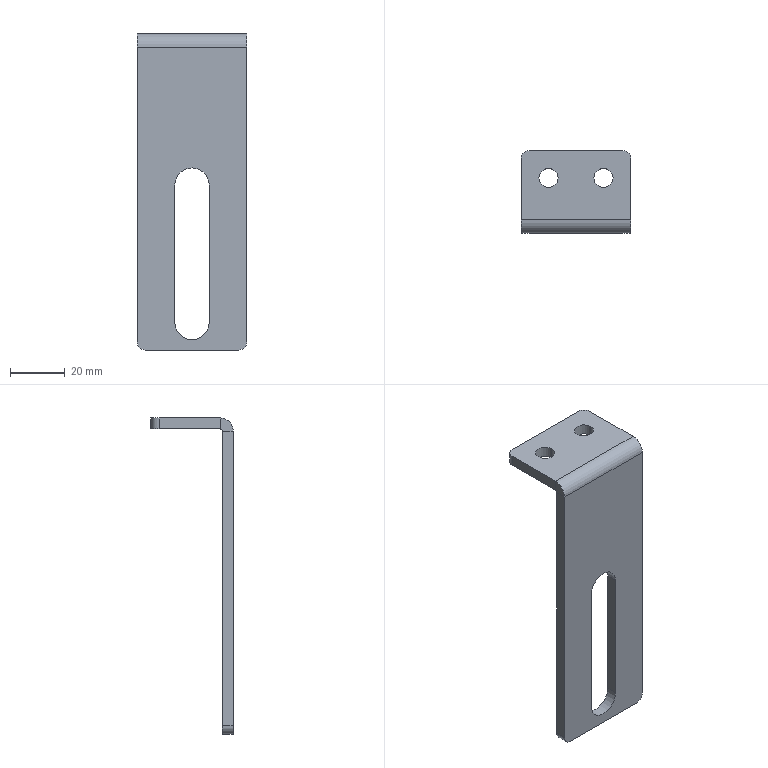Part | SolidWorks | features BaseBody 1 | 1 solid | 27 faces | box 40 x 30 x 115 mm | volume 19042 mm3 | plane 14 | cylinder 13 | commonest cylinder face diameters 6 x4 7 x4 12.5 x3 1.473 x1 9.473 x1
STEP:
#1=CARTESIAN_POINT('',(6.25,-15.,-55.));
#2=VERTEX_POINT('',#1);
#3=CARTESIAN_POINT('',(0.,-15.,-48.75));
#4=VERTEX_POINT('',#3);
#5=CARTESIAN_POINT('',(0.,-15.,-55.));
#6=DIRECTION('',(0.,-1.,0.));
#7=DIRECTION('',(0.,0.,-1.));
#8=AXIS2_PLACEMENT_3D('',#5,#6,#7);
#9=CIRCLE('',#8,6.25);
#10=EDGE_CURVE('',#2,#4,#9,.T.);
#11=ORIENTED_EDGE('',*,*,#10,.T.);
#12=CARTESIAN_POINT('',(0.,-11.,-48.75));
#13=VERTEX_POINT('',#12);
#14=CARTESIAN_POINT('',(0.,-21.,-48.75));
#15=DIRECTION('',(0.,1.,0.));
#16=VECTOR('',#15,1000.);
#17=LINE('',#14,#16);
#18=EDGE_CURVE('',#4,#13,#17,.T.);
#19=ORIENTED_EDGE('',*,*,#18,.T.);
#20=CARTESIAN_POINT('',(6.25,-11.,-55.));
#21=VERTEX_POINT('',#20);
#22=CARTESIAN_POINT('',(0.,-11.,-55.));
#23=DIRECTION('',(0.,1.,0.));
#24=DIRECTION('',(0.,0.,1.));
#25=AXIS2_PLACEMENT_3D('',#22,#23,#24);
#26=CIRCLE('',#25,6.25);
#27=EDGE_CURVE('',#13,#21,#26,.T.);
#28=ORIENTED_EDGE('',*,*,#27,.T.);
#29=CARTESIAN_POINT('',(6.25,-21.,-55.));
#30=DIRECTION('',(0.,1.,0.));
#31=VECTOR('',#30,1000.);
#32=LINE('',#29,#31);
#33=EDGE_CURVE('',#2,#21,#32,.T.);
#34=ORIENTED_EDGE('',*,*,#33,.F.);
#35=EDGE_LOOP('',(#11,#19,#28,#34));
#36=FACE_OUTER_BOUND('',#35,.T.);
#37=CARTESIAN_POINT('',(0.,-21.,-55.));
#38=DIRECTION('',(0.,1.,0.));
#39=DIRECTION('',(0.,0.,1.));
#40=AXIS2_PLACEMENT_3D('',#37,#38,#39);
#41=CYLINDRICAL_SURFACE('',#40,6.25);
#42=ADVANCED_FACE('',(#36),#41,.F.);
#43=CARTESIAN_POINT('',(-13.5,5.,-4.));
#44=VERTEX_POINT('',#43);
#45=CARTESIAN_POINT('',(-6.5,5.,-4.));
#46=VERTEX_POINT('',#45);
#47=CARTESIAN_POINT('',(-10.,5.,-4.));
#48=DIRECTION('',(0.,0.,1.));
#49=DIRECTION('',(1.,0.,0.));
#50=AXIS2_PLACEMENT_3D('',#47,#48,#49);
#51=CIRCLE('',#50,3.5);
#52=EDGE_CURVE('',#44,#46,#51,.T.);
#53=ORIENTED_EDGE('',*,*,#52,.F.);
#54=CARTESIAN_POINT('',(-13.5,5.,0.));
#55=VERTEX_POINT('',#54);
#56=CARTESIAN_POINT('',(-13.5,5.,0.));
#57=DIRECTION('',(0.,0.,1.));
#58=VECTOR('',#57,1000.);
#59=LINE('',#56,#58);
#60=EDGE_CURVE('',#44,#55,#59,.T.);
#61=ORIENTED_EDGE('',*,*,#60,.T.);
#62=CARTESIAN_POINT('',(-6.5,5.,0.));
#63=VERTEX_POINT('',#62);
#64=CARTESIAN_POINT('',(-10.,5.,0.));
#65=DIRECTION('',(0.,0.,1.));
#66=DIRECTION('',(1.,0.,0.));
#67=AXIS2_PLACEMENT_3D('',#64,#65,#66);
#68=CIRCLE('',#67,3.5);
#69=EDGE_CURVE('',#55,#63,#68,.T.);
#70=ORIENTED_EDGE('',*,*,#69,.T.);
#71=CARTESIAN_POINT('',(-6.5,5.,0.));
#72=DIRECTION('',(0.,0.,1.));
#73=VECTOR('',#72,1000.);
#74=LINE('',#71,#73);
#75=EDGE_CURVE('',#46,#63,#74,.T.);
#76=ORIENTED_EDGE('',*,*,#75,.F.);
#77=EDGE_LOOP('',(#53,#61,#70,#76));
#78=FACE_OUTER_BOUND('',#77,.T.);
#79=CARTESIAN_POINT('',(-10.,5.,0.));
#80=DIRECTION('',(0.,0.,1.));
#81=DIRECTION('',(1.,0.,0.));
#82=AXIS2_PLACEMENT_3D('',#79,#80,#81);
#83=CYLINDRICAL_SURFACE('',#82,3.5);
#84=ADVANCED_FACE('',(#78),#83,.F.);
#85=CARTESIAN_POINT('',(6.5,5.,-4.));
#86=VERTEX_POINT('',#85);
#87=CARTESIAN_POINT('',(13.5,5.,-4.));
#88=VERTEX_POINT('',#87);
#89=CARTESIAN_POINT('',(10.,5.,-4.));
#90=DIRECTION('',(0.,0.,1.));
#91=DIRECTION('',(1.,0.,0.));
#92=AXIS2_PLACEMENT_3D('',#89,#90,#91);
#93=CIRCLE('',#92,3.5);
#94=EDGE_CURVE('',#86,#88,#93,.T.);
#95=ORIENTED_EDGE('',*,*,#94,.F.);
#96=CARTESIAN_POINT('',(6.5,5.,0.));
#97=VERTEX_POINT('',#96);
#98=CARTESIAN_POINT('',(6.5,5.,0.));
#99=DIRECTION('',(0.,0.,1.));
#100=VECTOR('',#99,1000.);
#101=LINE('',#98,#100);
#102=EDGE_CURVE('',#86,#97,#101,.T.);
#103=ORIENTED_EDGE('',*,*,#102,.T.);
#104=CARTESIAN_POINT('',(13.5,5.,0.));
#105=VERTEX_POINT('',#104);
#106=CARTESIAN_POINT('',(10.,5.,0.));
#107=DIRECTION('',(0.,0.,1.));
#108=DIRECTION('',(1.,0.,0.));
#109=AXIS2_PLACEMENT_3D('',#106,#107,#108);
#110=CIRCLE('',#109,3.5);
#111=EDGE_CURVE('',#97,#105,#110,.T.);
#112=ORIENTED_EDGE('',*,*,#111,.T.);
#113=CARTESIAN_POINT('',(13.5,5.,0.));
#114=DIRECTION('',(0.,0.,1.));
#115=VECTOR('',#114,1000.);
#116=LINE('',#113,#115);
#117=EDGE_CURVE('',#88,#105,#116,.T.);
#118=ORIENTED_EDGE('',*,*,#117,.F.);
#119=EDGE_LOOP('',(#95,#103,#112,#118));
#120=FACE_OUTER_BOUND('',#119,.T.);
#121=CARTESIAN_POINT('',(10.,5.,0.));
#122=DIRECTION('',(0.,0.,1.));
#123=DIRECTION('',(1.,0.,0.));
#124=AXIS2_PLACEMENT_3D('',#121,#122,#123);
#125=CYLINDRICAL_SURFACE('',#124,3.5);
#126=ADVANCED_FACE('',(#120),#125,.F.);
#127=CARTESIAN_POINT('',(-20.,12.,0.));
#128=VERTEX_POINT('',#127);
#129=CARTESIAN_POINT('',(-20.,-10.263,0.));
#130=VERTEX_POINT('',#129);
#131=CARTESIAN_POINT('',(-20.,15.,0.));
#132=DIRECTION('',(0.,-1.,0.));
#133=VECTOR('',#132,1000.);
#134=LINE('',#131,#133);
#135=EDGE_CURVE('',#128,#130,#134,.T.);
#136=ORIENTED_EDGE('',*,*,#135,.F.);
#137=CARTESIAN_POINT('',(-20.,12.,-4.));
#138=VERTEX_POINT('',#137);
#139=CARTESIAN_POINT('',(-20.,12.,-4.));
#140=DIRECTION('',(0.,0.,-1.));
#141=VECTOR('',#140,1000.);
#142=LINE('',#139,#141);
#143=EDGE_CURVE('',#128,#138,#142,.T.);
#144=ORIENTED_EDGE('',*,*,#143,.T.);
#145=CARTESIAN_POINT('',(-20.,-10.263,-4.));
#146=VERTEX_POINT('',#145);
#147=CARTESIAN_POINT('',(-20.,15.,-4.));
#148=DIRECTION('',(0.,-1.,0.));
#149=VECTOR('',#148,1000.);
#150=LINE('',#147,#149);
#151=EDGE_CURVE('',#138,#146,#150,.T.);
#152=ORIENTED_EDGE('',*,*,#151,.T.);
#153=CARTESIAN_POINT('',(-20.,-10.263,-4.));
#154=DIRECTION('',(0.,0.,1.));
#155=VECTOR('',#154,1000.);
#156=LINE('',#153,#155);
#157=EDGE_CURVE('',#146,#130,#156,.T.);
#158=ORIENTED_EDGE('',*,*,#157,.T.);
#159=EDGE_LOOP('',(#136,#144,#152,#158));
#160=FACE_OUTER_BOUND('',#159,.T.);
#161=CARTESIAN_POINT('',(-20.,15.,-4.));
#162=DIRECTION('',(-1.,0.,0.));
#163=DIRECTION('',(0.,-1.,0.));
#164=AXIS2_PLACEMENT_3D('',#161,#162,#163);
#165=PLANE('',#164);
#166=ADVANCED_FACE('',(#160),#165,.T.);
#167=CARTESIAN_POINT('',(-10.,5.,-4.));
#168=DIRECTION('',(0.,0.,1.));
#169=DIRECTION('',(1.,0.,0.));
#170=AXIS2_PLACEMENT_3D('',#167,#168,#169);
#171=CIRCLE('',#170,3.5);
#172=EDGE_CURVE('',#46,#44,#171,.T.);
#173=ORIENTED_EDGE('',*,*,#172,.T.);
#174=ORIENTED_EDGE('',*,*,#52,.T.);
#175=EDGE_LOOP('',(#173,#174));
#176=FACE_BOUND('',#175,.T.);
#177=CARTESIAN_POINT('',(10.,5.,-4.));
#178=DIRECTION('',(0.,0.,1.));
#179=DIRECTION('',(1.,0.,0.));
#180=AXIS2_PLACEMENT_3D('',#177,#178,#179);
#181=CIRCLE('',#180,3.5);
#182=EDGE_CURVE('',#88,#86,#181,.T.);
#183=ORIENTED_EDGE('',*,*,#182,.T.);
#184=ORIENTED_EDGE('',*,*,#94,.T.);
#185=EDGE_LOOP('',(#183,#184));
#186=FACE_BOUND('',#185,.T.);
#187=CARTESIAN_POINT('',(17.,15.,-4.));
#188=VERTEX_POINT('',#187);
#189=CARTESIAN_POINT('',(-17.,15.,-4.));
#190=VERTEX_POINT('',#189);
#191=CARTESIAN_POINT('',(-20.,15.,-4.));
#192=DIRECTION('',(-1.,0.,0.));
#193=VECTOR('',#192,1000.);
#194=LINE('',#191,#193);
#195=EDGE_CURVE('',#188,#190,#194,.T.);
#196=ORIENTED_EDGE('',*,*,#195,.F.);
#197=CARTESIAN_POINT('',(20.,12.,-4.));
#198=VERTEX_POINT('',#197);
#199=CARTESIAN_POINT('',(17.,12.,-4.));
#200=DIRECTION('',(0.,0.,-1.));
#201=DIRECTION('',(1.,0.,0.));
#202=AXIS2_PLACEMENT_3D('',#199,#200,#201);
#203=CIRCLE('',#202,3.);
#204=EDGE_CURVE('',#188,#198,#203,.T.);
#205=ORIENTED_EDGE('',*,*,#204,.T.);
#206=CARTESIAN_POINT('',(20.,-10.263,-4.));
#207=VERTEX_POINT('',#206);
#208=CARTESIAN_POINT('',(20.,15.,-4.));
#209=DIRECTION('',(0.,1.,0.));
#210=VECTOR('',#209,1000.);
#211=LINE('',#208,#210);
#212=EDGE_CURVE('',#207,#198,#211,.T.);
#213=ORIENTED_EDGE('',*,*,#212,.F.);
#214=CARTESIAN_POINT('',(-20.,-10.263,-4.));
#215=DIRECTION('',(1.,0.,0.));
#216=VECTOR('',#215,1000.);
#217=LINE('',#214,#216);
#218=EDGE_CURVE('',#146,#207,#217,.T.);
#219=ORIENTED_EDGE('',*,*,#218,.F.);
#220=ORIENTED_EDGE('',*,*,#151,.F.);
#221=CARTESIAN_POINT('',(-17.,12.,-4.));
#222=DIRECTION('',(0.,0.,-1.));
#223=DIRECTION('',(1.,0.,0.));
#224=AXIS2_PLACEMENT_3D('',#221,#222,#223);
#225=CIRCLE('',#224,3.);
#226=EDGE_CURVE('',#138,#190,#225,.T.);
#227=ORIENTED_EDGE('',*,*,#226,.T.);
#228=EDGE_LOOP('',(#196,#205,#213,#219,#220,#227));
#229=FACE_OUTER_BOUND('',#228,.T.);
#230=CARTESIAN_POINT('',(0.,0.,-4.));
#231=DIRECTION('',(0.,0.,1.));
#232=DIRECTION('',(1.,0.,0.));
#233=AXIS2_PLACEMENT_3D('',#230,#231,#232);
#234=PLANE('',#233);
#235=ADVANCED_FACE('',(#176,#186,#229),#234,.F.);
#236=CARTESIAN_POINT('',(-10.,5.,0.));
#237=DIRECTION('',(0.,0.,1.));
#238=DIRECTION('',(1.,0.,0.));
#239=AXIS2_PLACEMENT_3D('',#236,#237,#238);
#240=CIRCLE('',#239,3.5);
#241=EDGE_CURVE('',#63,#55,#240,.T.);
#242=ORIENTED_EDGE('',*,*,#241,.F.);
#243=ORIENTED_EDGE('',*,*,#69,.F.);
#244=EDGE_LOOP('',(#242,#243));
#245=FACE_BOUND('',#244,.T.);
#246=CARTESIAN_POINT('',(10.,5.,0.));
#247=DIRECTION('',(0.,0.,1.));
#248=DIRECTION('',(1.,0.,0.));
#249=AXIS2_PLACEMENT_3D('',#246,#247,#248);
#250=CIRCLE('',#249,3.5);
#251=EDGE_CURVE('',#105,#97,#250,.T.);
#252=ORIENTED_EDGE('',*,*,#251,.F.);
#253=ORIENTED_EDGE('',*,*,#111,.F.);
#254=EDGE_LOOP('',(#252,#253));
#255=FACE_BOUND('',#254,.T.);
#256=CARTESIAN_POINT('',(20.,-10.263,0.));
#257=VERTEX_POINT('',#256);
#258=CARTESIAN_POINT('',(20.,12.,0.));
#259=VERTEX_POINT('',#258);
#260=CARTESIAN_POINT('',(20.,15.,0.));
#261=DIRECTION('',(0.,1.,0.));
#262=VECTOR('',#261,1000.);
#263=LINE('',#260,#262);
#264=EDGE_CURVE('',#257,#259,#263,.T.);
#265=ORIENTED_EDGE('',*,*,#264,.T.);
#266=CARTESIAN_POINT('',(17.,15.,0.));
#267=VERTEX_POINT('',#266);
#268=CARTESIAN_POINT('',(17.,12.,0.));
#269=DIRECTION('',(0.,0.,1.));
#270=DIRECTION('',(1.,0.,0.));
#271=AXIS2_PLACEMENT_3D('',#268,#269,#270);
#272=CIRCLE('',#271,3.);
#273=EDGE_CURVE('',#259,#267,#272,.T.);
#274=ORIENTED_EDGE('',*,*,#273,.T.);
#275=CARTESIAN_POINT('',(-17.,15.,0.));
#276=VERTEX_POINT('',#275);
#277=CARTESIAN_POINT('',(-20.,15.,0.));
#278=DIRECTION('',(-1.,0.,0.));
#279=VECTOR('',#278,1000.);
#280=LINE('',#277,#279);
#281=EDGE_CURVE('',#267,#276,#280,.T.);
#282=ORIENTED_EDGE('',*,*,#281,.T.);
#283=CARTESIAN_POINT('',(-17.,12.,0.));
#284=DIRECTION('',(0.,0.,1.));
#285=DIRECTION('',(1.,0.,0.));
#286=AXIS2_PLACEMENT_3D('',#283,#284,#285);
#287=CIRCLE('',#286,3.);
#288=EDGE_CURVE('',#276,#128,#287,.T.);
#289=ORIENTED_EDGE('',*,*,#288,.T.);
#290=ORIENTED_EDGE('',*,*,#135,.T.);
#291=CARTESIAN_POINT('',(-20.,-10.263,0.));
#292=DIRECTION('',(1.,0.,0.));
#293=VECTOR('',#292,1000.);
#294=LINE('',#291,#293);
#295=EDGE_CURVE('',#130,#257,#294,.T.);
#296=ORIENTED_EDGE('',*,*,#295,.T.);
#297=EDGE_LOOP('',(#265,#274,#282,#289,#290,#296));
#298=FACE_OUTER_BOUND('',#297,.T.);
#299=CARTESIAN_POINT('',(0.,0.,0.));
#300=DIRECTION('',(0.,0.,1.));
#301=DIRECTION('',(1.,0.,0.));
#302=AXIS2_PLACEMENT_3D('',#299,#300,#301);
#303=PLANE('',#302);
#304=ADVANCED_FACE('',(#245,#255,#298),#303,.T.);
#305=ORIENTED_EDGE('',*,*,#212,.T.);
#306=CARTESIAN_POINT('',(20.,12.,-4.));
#307=DIRECTION('',(0.,0.,1.));
#308=VECTOR('',#307,1000.);
#309=LINE('',#306,#308);
#310=EDGE_CURVE('',#198,#259,#309,.T.);
#311=ORIENTED_EDGE('',*,*,#310,.T.);
#312=ORIENTED_EDGE('',*,*,#264,.F.);
#313=CARTESIAN_POINT('',(20.,-10.263,-4.));
#314=DIRECTION('',(0.,0.,1.));
#315=VECTOR('',#314,1000.);
#316=LINE('',#313,#315);
#317=EDGE_CURVE('',#207,#257,#316,.T.);
#318=ORIENTED_EDGE('',*,*,#317,.F.);
#319=EDGE_LOOP('',(#305,#311,#312,#318));
#320=FACE_OUTER_BOUND('',#319,.T.);
#321=CARTESIAN_POINT('',(20.,15.,-4.));
#322=DIRECTION('',(1.,0.,0.));
#323=DIRECTION('',(0.,1.,0.));
#324=AXIS2_PLACEMENT_3D('',#321,#322,#323);
#325=PLANE('',#324);
#326=ADVANCED_FACE('',(#320),#325,.T.);
#327=ORIENTED_EDGE('',*,*,#281,.F.);
#328=CARTESIAN_POINT('',(17.,15.,-4.));
#329=DIRECTION('',(0.,0.,-1.));
#330=VECTOR('',#329,1000.);
#331=LINE('',#328,#330);
#332=EDGE_CURVE('',#267,#188,#331,.T.);
#333=ORIENTED_EDGE('',*,*,#332,.T.);
#334=ORIENTED_EDGE('',*,*,#195,.T.);
#335=CARTESIAN_POINT('',(-17.,15.,-4.));
#336=DIRECTION('',(0.,0.,1.));
#337=VECTOR('',#336,1000.);
#338=LINE('',#335,#337);
#339=EDGE_CURVE('',#190,#276,#338,.T.);
#340=ORIENTED_EDGE('',*,*,#339,.T.);
#341=EDGE_LOOP('',(#327,#333,#334,#340));
#342=FACE_OUTER_BOUND('',#341,.T.);
#343=CARTESIAN_POINT('',(-20.,15.,-4.));
#344=DIRECTION('',(0.,1.,0.));
#345=DIRECTION('',(0.,0.,1.));
#346=AXIS2_PLACEMENT_3D('',#343,#344,#345);
#347=PLANE('',#346);
#348=ADVANCED_FACE('',(#342),#347,.T.);
#349=CARTESIAN_POINT('',(20.,-11.,-4.737));
#350=VERTEX_POINT('',#349);
#351=CARTESIAN_POINT('',(20.,-15.,-4.737));
#352=VERTEX_POINT('',#351);
#353=CARTESIAN_POINT('',(20.,-15.,-4.737));
#354=DIRECTION('',(0.,-1.,0.));
#355=VECTOR('',#354,1000.);
#356=LINE('',#353,#355);
#357=EDGE_CURVE('',#350,#352,#356,.T.);
#358=ORIENTED_EDGE('',*,*,#357,.F.);
#359=CARTESIAN_POINT('',(20.,-10.263,-4.737));
#360=DIRECTION('',(1.,0.,0.));
#361=DIRECTION('',(0.,0.,1.));
#362=AXIS2_PLACEMENT_3D('',#359,#360,#361);
#363=CIRCLE('',#362,0.7366);
#364=EDGE_CURVE('',#207,#350,#363,.T.);
#365=ORIENTED_EDGE('',*,*,#364,.F.);
#366=ORIENTED_EDGE('',*,*,#317,.T.);
#367=CARTESIAN_POINT('',(20.,-10.263,-4.737));
#368=DIRECTION('',(1.,0.,0.));
#369=DIRECTION('',(0.,0.,1.));
#370=AXIS2_PLACEMENT_3D('',#367,#368,#369);
#371=CIRCLE('',#370,4.737);
#372=EDGE_CURVE('',#257,#352,#371,.T.);
#373=ORIENTED_EDGE('',*,*,#372,.T.);
#374=EDGE_LOOP('',(#358,#365,#366,#373));
#375=FACE_OUTER_BOUND('',#374,.T.);
#376=CARTESIAN_POINT('',(20.,-10.263,-4.737));
#377=DIRECTION('',(1.,0.,0.));
#378=DIRECTION('',(0.,0.,-1.));
#379=AXIS2_PLACEMENT_3D('',#376,#377,#378);
#380=PLANE('',#379);
#381=ADVANCED_FACE('',(#375),#380,.T.);
#382=CARTESIAN_POINT('',(-20.,-11.,-4.737));
#383=VERTEX_POINT('',#382);
#384=CARTESIAN_POINT('',(-20.,-10.263,-4.737));
#385=DIRECTION('',(-1.,0.,0.));
#386=DIRECTION('',(0.,0.,1.));
#387=AXIS2_PLACEMENT_3D('',#384,#385,#386);
#388=CIRCLE('',#387,0.7366);
#389=EDGE_CURVE('',#383,#146,#388,.T.);
#390=ORIENTED_EDGE('',*,*,#389,.F.);
#391=CARTESIAN_POINT('',(-20.,-15.,-4.737));
#392=VERTEX_POINT('',#391);
#393=CARTESIAN_POINT('',(-20.,-11.,-4.737));
#394=DIRECTION('',(0.,-1.,0.));
#395=VECTOR('',#394,1000.);
#396=LINE('',#393,#395);
#397=EDGE_CURVE('',#383,#392,#396,.T.);
#398=ORIENTED_EDGE('',*,*,#397,.T.);
#399=CARTESIAN_POINT('',(-20.,-10.263,-4.737));
#400=DIRECTION('',(-1.,0.,0.));
#401=DIRECTION('',(0.,0.,1.));
#402=AXIS2_PLACEMENT_3D('',#399,#400,#401);
#403=CIRCLE('',#402,4.737);
#404=EDGE_CURVE('',#392,#130,#403,.T.);
#405=ORIENTED_EDGE('',*,*,#404,.T.);
#406=ORIENTED_EDGE('',*,*,#157,.F.);
#407=EDGE_LOOP('',(#390,#398,#405,#406));
#408=FACE_OUTER_BOUND('',#407,.T.);
#409=CARTESIAN_POINT('',(-20.,-10.263,-4.737));
#410=DIRECTION('',(1.,0.,0.));
#411=DIRECTION('',(0.,0.,-1.));
#412=AXIS2_PLACEMENT_3D('',#409,#410,#411);
#413=PLANE('',#412);
#414=ADVANCED_FACE('',(#408),#413,.F.);
#415=ORIENTED_EDGE('',*,*,#295,.F.);
#416=ORIENTED_EDGE('',*,*,#404,.F.);
#417=CARTESIAN_POINT('',(0.,-15.,-4.737));
#418=DIRECTION('',(-1.,0.,0.));
#419=VECTOR('',#418,1000.);
#420=LINE('',#417,#419);
#421=EDGE_CURVE('',#352,#392,#420,.T.);
#422=ORIENTED_EDGE('',*,*,#421,.F.);
#423=ORIENTED_EDGE('',*,*,#372,.F.);
#424=EDGE_LOOP('',(#415,#416,#422,#423));
#425=FACE_OUTER_BOUND('',#424,.T.);
#426=CARTESIAN_POINT('',(-20.,-10.263,-4.737));
#427=DIRECTION('',(-1.,0.,0.));
#428=DIRECTION('',(0.,-1.,0.));
#429=AXIS2_PLACEMENT_3D('',#426,#427,#428);
#430=CYLINDRICAL_SURFACE('',#429,4.737);
#431=ADVANCED_FACE('',(#425),#430,.T.);
#432=ORIENTED_EDGE('',*,*,#218,.T.);
#433=ORIENTED_EDGE('',*,*,#364,.T.);
#434=CARTESIAN_POINT('',(20.,-11.,-4.737));
#435=DIRECTION('',(-1.,0.,0.));
#436=VECTOR('',#435,1000.);
#437=LINE('',#434,#436);
#438=EDGE_CURVE('',#350,#383,#437,.T.);
#439=ORIENTED_EDGE('',*,*,#438,.T.);
#440=ORIENTED_EDGE('',*,*,#389,.T.);
#441=EDGE_LOOP('',(#432,#433,#439,#440));
#442=FACE_OUTER_BOUND('',#441,.T.);
#443=CARTESIAN_POINT('',(-20.,-10.263,-4.737));
#444=DIRECTION('',(-1.,0.,0.));
#445=DIRECTION('',(0.,-1.,0.));
#446=AXIS2_PLACEMENT_3D('',#443,#444,#445);
#447=CYLINDRICAL_SURFACE('',#446,0.7366);
#448=ADVANCED_FACE('',(#442),#447,.F.);
#449=CARTESIAN_POINT('',(-20.,-11.,-112.));
#450=VERTEX_POINT('',#449);
#451=CARTESIAN_POINT('',(-20.,-11.,0.));
#452=DIRECTION('',(0.,0.,1.));
#453=VECTOR('',#452,1000.);
#454=LINE('',#451,#453);
#455=EDGE_CURVE('',#450,#383,#454,.T.);
#456=ORIENTED_EDGE('',*,*,#455,.F.);
#457=CARTESIAN_POINT('',(-20.,-15.,-112.));
#458=VERTEX_POINT('',#457);
#459=CARTESIAN_POINT('',(-20.,-15.,-112.));
#460=DIRECTION('',(0.,-1.,0.));
#461=VECTOR('',#460,1000.);
#462=LINE('',#459,#461);
#463=EDGE_CURVE('',#450,#458,#462,.T.);
#464=ORIENTED_EDGE('',*,*,#463,.T.);
#465=CARTESIAN_POINT('',(-20.,-15.,-4.));
#466=DIRECTION('',(0.,0.,1.));
#467=VECTOR('',#466,1000.);
#468=LINE('',#465,#467);
#469=EDGE_CURVE('',#458,#392,#468,.T.);
#470=ORIENTED_EDGE('',*,*,#469,.T.);
#471=ORIENTED_EDGE('',*,*,#397,.F.);
#472=EDGE_LOOP('',(#456,#464,#470,#471));
#473=FACE_OUTER_BOUND('',#472,.T.);
#474=CARTESIAN_POINT('',(-20.,-15.,-4.));
#475=DIRECTION('',(-1.,0.,0.));
#476=DIRECTION('',(0.,0.,1.));
#477=AXIS2_PLACEMENT_3D('',#474,#475,#476);
#478=PLANE('',#477);
#479=ADVANCED_FACE('',(#473),#478,.T.);
#480=CARTESIAN_POINT('',(20.,-15.,-112.));
#481=VERTEX_POINT('',#480);
#482=CARTESIAN_POINT('',(20.,-15.,-115.));
#483=DIRECTION('',(0.,0.,-1.));
#484=VECTOR('',#483,1000.);
#485=LINE('',#482,#484);
#486=EDGE_CURVE('',#352,#481,#485,.T.);
#487=ORIENTED_EDGE('',*,*,#486,.T.);
#488=CARTESIAN_POINT('',(20.,-11.,-112.));
#489=VERTEX_POINT('',#488);
#490=CARTESIAN_POINT('',(20.,-15.,-112.));
#491=DIRECTION('',(0.,1.,0.));
#492=VECTOR('',#491,1000.);
#493=LINE('',#490,#492);
#494=EDGE_CURVE('',#481,#489,#493,.T.);
#495=ORIENTED_EDGE('',*,*,#494,.T.);
#496=CARTESIAN_POINT('',(20.,-11.,0.));
#497=DIRECTION('',(0.,0.,-1.));
#498=VECTOR('',#497,1000.);
#499=LINE('',#496,#498);
#500=EDGE_CURVE('',#350,#489,#499,.T.);
#501=ORIENTED_EDGE('',*,*,#500,.F.);
#502=ORIENTED_EDGE('',*,*,#357,.T.);
#503=EDGE_LOOP('',(#487,#495,#501,#502));
#504=FACE_OUTER_BOUND('',#503,.T.);
#505=CARTESIAN_POINT('',(20.,-15.,-115.));
#506=DIRECTION('',(1.,0.,0.));
#507=DIRECTION('',(0.,0.,-1.));
#508=AXIS2_PLACEMENT_3D('',#505,#506,#507);
#509=PLANE('',#508);
#510=ADVANCED_FACE('',(#504),#509,.T.);
#511=CARTESIAN_POINT('',(-6.25,-15.,-105.));
#512=VERTEX_POINT('',#511);
#513=CARTESIAN_POINT('',(6.25,-15.,-105.));
#514=VERTEX_POINT('',#513);
#515=CARTESIAN_POINT('',(0.,-15.,-105.));
#516=DIRECTION('',(0.,-1.,0.));
#517=DIRECTION('',(0.,0.,-1.));
#518=AXIS2_PLACEMENT_3D('',#515,#516,#517);
#519=CIRCLE('',#518,6.25);
#520=EDGE_CURVE('',#512,#514,#519,.T.);
#521=ORIENTED_EDGE('',*,*,#520,.F.);
#522=CARTESIAN_POINT('',(-6.25,-15.,-55.));
#523=VERTEX_POINT('',#522);
#524=CARTESIAN_POINT('',(-6.25,-15.,0.));
#525=DIRECTION('',(0.,0.,-1.));
#526=VECTOR('',#525,1000.);
#527=LINE('',#524,#526);
#528=EDGE_CURVE('',#523,#512,#527,.T.);
#529=ORIENTED_EDGE('',*,*,#528,.F.);
#530=CARTESIAN_POINT('',(0.,-15.,-55.));
#531=DIRECTION('',(0.,-1.,0.));
#532=DIRECTION('',(0.,0.,-1.));
#533=AXIS2_PLACEMENT_3D('',#530,#531,#532);
#534=CIRCLE('',#533,6.25);
#535=EDGE_CURVE('',#4,#523,#534,.T.);
#536=ORIENTED_EDGE('',*,*,#535,.F.);
#537=ORIENTED_EDGE('',*,*,#10,.F.);
#538=CARTESIAN_POINT('',(6.25,-15.,0.));
#539=DIRECTION('',(0.,0.,1.));
#540=VECTOR('',#539,1000.);
#541=LINE('',#538,#540);
#542=EDGE_CURVE('',#514,#2,#541,.T.);
#543=ORIENTED_EDGE('',*,*,#542,.F.);
#544=EDGE_LOOP('',(#521,#529,#536,#537,#543));
#545=FACE_BOUND('',#544,.T.);
#546=ORIENTED_EDGE('',*,*,#469,.F.);
#547=CARTESIAN_POINT('',(-17.,-15.,-115.));
#548=VERTEX_POINT('',#547);
#549=CARTESIAN_POINT('',(-17.,-15.,-112.));
#550=DIRECTION('',(0.,-1.,0.));
#551=DIRECTION('',(0.,0.,-1.));
#552=AXIS2_PLACEMENT_3D('',#549,#550,#551);
#553=CIRCLE('',#552,3.);
#554=EDGE_CURVE('',#458,#548,#553,.T.);
#555=ORIENTED_EDGE('',*,*,#554,.T.);
#556=CARTESIAN_POINT('',(17.,-15.,-115.));
#557=VERTEX_POINT('',#556);
#558=CARTESIAN_POINT('',(-20.,-15.,-115.));
#559=DIRECTION('',(-1.,0.,0.));
#560=VECTOR('',#559,1000.);
#561=LINE('',#558,#560);
#562=EDGE_CURVE('',#557,#548,#561,.T.);
#563=ORIENTED_EDGE('',*,*,#562,.F.);
#564=CARTESIAN_POINT('',(17.,-15.,-112.));
#565=DIRECTION('',(0.,-1.,0.));
#566=DIRECTION('',(0.,0.,-1.));
#567=AXIS2_PLACEMENT_3D('',#564,#565,#566);
#568=CIRCLE('',#567,3.);
#569=EDGE_CURVE('',#557,#481,#568,.T.);
#570=ORIENTED_EDGE('',*,*,#569,.T.);
#571=ORIENTED_EDGE('',*,*,#486,.F.);
#572=ORIENTED_EDGE('',*,*,#421,.T.);
#573=EDGE_LOOP('',(#546,#555,#563,#570,#571,#572));
#574=FACE_OUTER_BOUND('',#573,.T.);
#575=CARTESIAN_POINT('',(0.,-15.,0.));
#576=DIRECTION('',(0.,-1.,0.));
#577=DIRECTION('',(0.,0.,-1.));
#578=AXIS2_PLACEMENT_3D('',#575,#576,#577);
#579=PLANE('',#578);
#580=ADVANCED_FACE('',(#545,#574),#579,.T.);
#581=CARTESIAN_POINT('',(-6.25,-11.,-105.));
#582=VERTEX_POINT('',#581);
#583=CARTESIAN_POINT('',(-6.25,-11.,-55.));
#584=VERTEX_POINT('',#583);
#585=CARTESIAN_POINT('',(-6.25,-11.,-105.));
#586=DIRECTION('',(0.,0.,1.));
#587=VECTOR('',#586,1000.);
#588=LINE('',#585,#587);
#589=EDGE_CURVE('',#582,#584,#588,.T.);
#590=ORIENTED_EDGE('',*,*,#589,.F.);
#591=CARTESIAN_POINT('',(6.25,-11.,-105.));
#592=VERTEX_POINT('',#591);
#593=CARTESIAN_POINT('',(0.,-11.,-105.));
#594=DIRECTION('',(0.,1.,0.));
#595=DIRECTION('',(0.,0.,1.));
#596=AXIS2_PLACEMENT_3D('',#593,#594,#595);
#597=CIRCLE('',#596,6.25);
#598=EDGE_CURVE('',#592,#582,#597,.T.);
#599=ORIENTED_EDGE('',*,*,#598,.F.);
#600=CARTESIAN_POINT('',(6.25,-11.,-105.));
#601=DIRECTION('',(0.,0.,-1.));
#602=VECTOR('',#601,1000.);
#603=LINE('',#600,#602);
#604=EDGE_CURVE('',#21,#592,#603,.T.);
#605=ORIENTED_EDGE('',*,*,#604,.F.);
#606=ORIENTED_EDGE('',*,*,#27,.F.);
#607=CARTESIAN_POINT('',(0.,-11.,-55.));
#608=DIRECTION('',(0.,1.,0.));
#609=DIRECTION('',(0.,0.,1.));
#610=AXIS2_PLACEMENT_3D('',#607,#608,#609);
#611=CIRCLE('',#610,6.25);
#612=EDGE_CURVE('',#584,#13,#611,.T.);
#613=ORIENTED_EDGE('',*,*,#612,.F.);
#614=EDGE_LOOP('',(#590,#599,#605,#606,#613));
#615=FACE_BOUND('',#614,.T.);
#616=CARTESIAN_POINT('',(17.,-11.,-115.));
#617=VERTEX_POINT('',#616);
#618=CARTESIAN_POINT('',(-17.,-11.,-115.));
#619=VERTEX_POINT('',#618);
#620=CARTESIAN_POINT('',(0.,-11.,-115.));
#621=DIRECTION('',(-1.,0.,0.));
#622=VECTOR('',#621,1000.);
#623=LINE('',#620,#622);
#624=EDGE_CURVE('',#617,#619,#623,.T.);
#625=ORIENTED_EDGE('',*,*,#624,.T.);
#626=CARTESIAN_POINT('',(-17.,-11.,-112.));
#627=DIRECTION('',(0.,1.,0.));
#628=DIRECTION('',(0.,0.,-1.));
#629=AXIS2_PLACEMENT_3D('',#626,#627,#628);
#630=CIRCLE('',#629,3.);
#631=EDGE_CURVE('',#619,#450,#630,.T.);
#632=ORIENTED_EDGE('',*,*,#631,.T.);
#633=ORIENTED_EDGE('',*,*,#455,.T.);
#634=ORIENTED_EDGE('',*,*,#438,.F.);
#635=ORIENTED_EDGE('',*,*,#500,.T.);
#636=CARTESIAN_POINT('',(17.,-11.,-112.));
#637=DIRECTION('',(0.,1.,0.));
#638=DIRECTION('',(0.,0.,-1.));
#639=AXIS2_PLACEMENT_3D('',#636,#637,#638);
#640=CIRCLE('',#639,3.);
#641=EDGE_CURVE('',#489,#617,#640,.T.);
#642=ORIENTED_EDGE('',*,*,#641,.T.);
#643=EDGE_LOOP('',(#625,#632,#633,#634,#635,#642));
#644=FACE_OUTER_BOUND('',#643,.T.);
#645=CARTESIAN_POINT('',(0.,-11.,0.));
#646=DIRECTION('',(0.,-1.,0.));
#647=DIRECTION('',(0.,0.,-1.));
#648=AXIS2_PLACEMENT_3D('',#645,#646,#647);
#649=PLANE('',#648);
#650=ADVANCED_FACE('',(#615,#644),#649,.F.);
#651=ORIENTED_EDGE('',*,*,#562,.T.);
#652=CARTESIAN_POINT('',(-17.,-15.,-115.));
#653=DIRECTION('',(0.,1.,0.));
#654=VECTOR('',#653,1000.);
#655=LINE('',#652,#654);
#656=EDGE_CURVE('',#548,#619,#655,.T.);
#657=ORIENTED_EDGE('',*,*,#656,.T.);
#658=ORIENTED_EDGE('',*,*,#624,.F.);
#659=CARTESIAN_POINT('',(17.,-15.,-115.));
#660=DIRECTION('',(0.,-1.,0.));
#661=VECTOR('',#660,1000.);
#662=LINE('',#659,#661);
#663=EDGE_CURVE('',#617,#557,#662,.T.);
#664=ORIENTED_EDGE('',*,*,#663,.T.);
#665=EDGE_LOOP('',(#651,#657,#658,#664));
#666=FACE_OUTER_BOUND('',#665,.T.);
#667=CARTESIAN_POINT('',(-20.,-15.,-115.));
#668=DIRECTION('',(0.,0.,-1.));
#669=DIRECTION('',(0.,1.,0.));
#670=AXIS2_PLACEMENT_3D('',#667,#668,#669);
#671=PLANE('',#670);
#672=ADVANCED_FACE('',(#666),#671,.T.);
#673=ORIENTED_EDGE('',*,*,#102,.F.);
#674=ORIENTED_EDGE('',*,*,#182,.F.);
#675=ORIENTED_EDGE('',*,*,#117,.T.);
#676=ORIENTED_EDGE('',*,*,#251,.T.);
#677=EDGE_LOOP('',(#673,#674,#675,#676));
#678=FACE_OUTER_BOUND('',#677,.T.);
#679=CARTESIAN_POINT('',(10.,5.,0.));
#680=DIRECTION('',(0.,0.,1.));
#681=DIRECTION('',(1.,0.,0.));
#682=AXIS2_PLACEMENT_3D('',#679,#680,#681);
#683=CYLINDRICAL_SURFACE('',#682,3.5);
#684=ADVANCED_FACE('',(#678),#683,.F.);
#685=ORIENTED_EDGE('',*,*,#60,.F.);
#686=ORIENTED_EDGE('',*,*,#172,.F.);
#687=ORIENTED_EDGE('',*,*,#75,.T.);
#688=ORIENTED_EDGE('',*,*,#241,.T.);
#689=EDGE_LOOP('',(#685,#686,#687,#688));
#690=FACE_OUTER_BOUND('',#689,.T.);
#691=CARTESIAN_POINT('',(-10.,5.,0.));
#692=DIRECTION('',(0.,0.,1.));
#693=DIRECTION('',(1.,0.,0.));
#694=AXIS2_PLACEMENT_3D('',#691,#692,#693);
#695=CYLINDRICAL_SURFACE('',#694,3.5);
#696=ADVANCED_FACE('',(#690),#695,.F.);
#697=ORIENTED_EDGE('',*,*,#554,.F.);
#698=ORIENTED_EDGE('',*,*,#463,.F.);
#699=ORIENTED_EDGE('',*,*,#631,.F.);
#700=ORIENTED_EDGE('',*,*,#656,.F.);
#701=EDGE_LOOP('',(#697,#698,#699,#700));
#702=FACE_OUTER_BOUND('',#701,.T.);
#703=CARTESIAN_POINT('',(-17.,-15.,-112.));
#704=DIRECTION('',(0.,1.,0.));
#705=DIRECTION('',(0.,0.,1.));
#706=AXIS2_PLACEMENT_3D('',#703,#704,#705);
#707=CYLINDRICAL_SURFACE('',#706,3.);
#708=ADVANCED_FACE('',(#702),#707,.T.);
#709=ORIENTED_EDGE('',*,*,#569,.F.);
#710=ORIENTED_EDGE('',*,*,#663,.F.);
#711=ORIENTED_EDGE('',*,*,#641,.F.);
#712=ORIENTED_EDGE('',*,*,#494,.F.);
#713=EDGE_LOOP('',(#709,#710,#711,#712));
#714=FACE_OUTER_BOUND('',#713,.T.);
#715=CARTESIAN_POINT('',(17.,-15.,-112.));
#716=DIRECTION('',(0.,1.,0.));
#717=DIRECTION('',(0.,0.,1.));
#718=AXIS2_PLACEMENT_3D('',#715,#716,#717);
#719=CYLINDRICAL_SURFACE('',#718,3.);
#720=ADVANCED_FACE('',(#714),#719,.T.);
#721=ORIENTED_EDGE('',*,*,#204,.F.);
#722=ORIENTED_EDGE('',*,*,#332,.F.);
#723=ORIENTED_EDGE('',*,*,#273,.F.);
#724=ORIENTED_EDGE('',*,*,#310,.F.);
#725=EDGE_LOOP('',(#721,#722,#723,#724));
#726=FACE_OUTER_BOUND('',#725,.T.);
#727=CARTESIAN_POINT('',(17.,12.,-4.));
#728=DIRECTION('',(0.,0.,1.));
#729=DIRECTION('',(1.,0.,0.));
#730=AXIS2_PLACEMENT_3D('',#727,#728,#729);
#731=CYLINDRICAL_SURFACE('',#730,3.);
#732=ADVANCED_FACE('',(#726),#731,.T.);
#733=ORIENTED_EDGE('',*,*,#226,.F.);
#734=ORIENTED_EDGE('',*,*,#143,.F.);
#735=ORIENTED_EDGE('',*,*,#288,.F.);
#736=ORIENTED_EDGE('',*,*,#339,.F.);
#737=EDGE_LOOP('',(#733,#734,#735,#736));
#738=FACE_OUTER_BOUND('',#737,.T.);
#739=CARTESIAN_POINT('',(-17.,12.,-4.));
#740=DIRECTION('',(0.,0.,1.));
#741=DIRECTION('',(1.,0.,0.));
#742=AXIS2_PLACEMENT_3D('',#739,#740,#741);
#743=CYLINDRICAL_SURFACE('',#742,3.);
#744=ADVANCED_FACE('',(#738),#743,.T.);
#745=ORIENTED_EDGE('',*,*,#520,.T.);
#746=CARTESIAN_POINT('',(6.25,-21.,-105.));
#747=DIRECTION('',(0.,1.,0.));
#748=VECTOR('',#747,1000.);
#749=LINE('',#746,#748);
#750=EDGE_CURVE('',#514,#592,#749,.T.);
#751=ORIENTED_EDGE('',*,*,#750,.T.);
#752=ORIENTED_EDGE('',*,*,#598,.T.);
#753=CARTESIAN_POINT('',(-6.25,-21.,-105.));
#754=DIRECTION('',(0.,1.,0.));
#755=VECTOR('',#754,1000.);
#756=LINE('',#753,#755);
#757=EDGE_CURVE('',#512,#582,#756,.T.);
#758=ORIENTED_EDGE('',*,*,#757,.F.);
#759=EDGE_LOOP('',(#745,#751,#752,#758));
#760=FACE_OUTER_BOUND('',#759,.T.);
#761=CARTESIAN_POINT('',(0.,-21.,-105.));
#762=DIRECTION('',(0.,1.,0.));
#763=DIRECTION('',(0.,0.,1.));
#764=AXIS2_PLACEMENT_3D('',#761,#762,#763);
#765=CYLINDRICAL_SURFACE('',#764,6.25);
#766=ADVANCED_FACE('',(#760),#765,.F.);
#767=ORIENTED_EDGE('',*,*,#542,.T.);
#768=ORIENTED_EDGE('',*,*,#33,.T.);
#769=ORIENTED_EDGE('',*,*,#604,.T.);
#770=ORIENTED_EDGE('',*,*,#750,.F.);
#771=EDGE_LOOP('',(#767,#768,#769,#770));
#772=FACE_OUTER_BOUND('',#771,.T.);
#773=CARTESIAN_POINT('',(6.25,-21.,-105.));
#774=DIRECTION('',(1.,0.,0.));
#775=DIRECTION('',(0.,0.,-1.));
#776=AXIS2_PLACEMENT_3D('',#773,#774,#775);
#777=PLANE('',#776);
#778=ADVANCED_FACE('',(#772),#777,.F.);
#779=ORIENTED_EDGE('',*,*,#18,.F.);
#780=ORIENTED_EDGE('',*,*,#535,.T.);
#781=CARTESIAN_POINT('',(-6.25,-21.,-55.));
#782=DIRECTION('',(0.,1.,0.));
#783=VECTOR('',#782,1000.);
#784=LINE('',#781,#783);
#785=EDGE_CURVE('',#523,#584,#784,.T.);
#786=ORIENTED_EDGE('',*,*,#785,.T.);
#787=ORIENTED_EDGE('',*,*,#612,.T.);
#788=EDGE_LOOP('',(#779,#780,#786,#787));
#789=FACE_OUTER_BOUND('',#788,.T.);
#790=CARTESIAN_POINT('',(0.,-21.,-55.));
#791=DIRECTION('',(0.,1.,0.));
#792=DIRECTION('',(0.,0.,1.));
#793=AXIS2_PLACEMENT_3D('',#790,#791,#792);
#794=CYLINDRICAL_SURFACE('',#793,6.25);
#795=ADVANCED_FACE('',(#789),#794,.F.);
#796=ORIENTED_EDGE('',*,*,#528,.T.);
#797=ORIENTED_EDGE('',*,*,#757,.T.);
#798=ORIENTED_EDGE('',*,*,#589,.T.);
#799=ORIENTED_EDGE('',*,*,#785,.F.);
#800=EDGE_LOOP('',(#796,#797,#798,#799));
#801=FACE_OUTER_BOUND('',#800,.T.);
#802=CARTESIAN_POINT('',(-6.25,-21.,-105.));
#803=DIRECTION('',(-1.,0.,0.));
#804=DIRECTION('',(0.,0.,1.));
#805=AXIS2_PLACEMENT_3D('',#802,#803,#804);
#806=PLANE('',#805);
#807=ADVANCED_FACE('',(#801),#806,.F.);
#808=CLOSED_SHELL('',(#42,#84,#126,#166,#235,#304,#326,#348,#381,#414,#431,#448,#479,#510,#580,#650,#672,#684,#696,#708,#720,#732,#744,#766,#778,#795,#807));
#809=MANIFOLD_SOLID_BREP('',#808);
#810=CARTESIAN_POINT('',(0.,0.,0.));
#811=DIRECTION('',(0.,0.,1.));
#812=DIRECTION('',(1.,0.,0.));
#813=AXIS2_PLACEMENT_3D('',#810,#811,#812);
#814=(LENGTH_UNIT()NAMED_UNIT(*)SI_UNIT(.MILLI.,.METRE.));
#815=UNCERTAINTY_MEASURE_WITH_UNIT(LENGTH_MEASURE(0.00001),#814,'','');
#816=(NAMED_UNIT(*)PLANE_ANGLE_UNIT()SI_UNIT($,.RADIAN.));
#817=(NAMED_UNIT(*)SI_UNIT($,.STERADIAN.)SOLID_ANGLE_UNIT());
#818=(GEOMETRIC_REPRESENTATION_CONTEXT(3)GLOBAL_UNCERTAINTY_ASSIGNED_CONTEXT((#815))GLOBAL_UNIT_ASSIGNED_CONTEXT((#814,#816,#817))REPRESENTATION_CONTEXT('',''));
#819=ADVANCED_BREP_SHAPE_REPRESENTATION('',(#809,#813),#818);